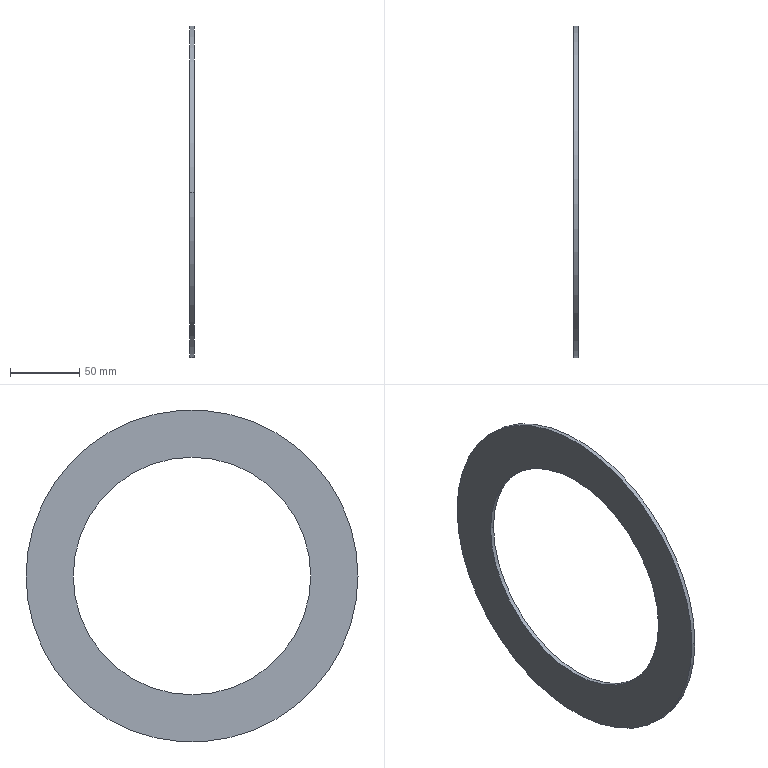Part | STEP file | 1 solid | 6 faces | box 3 x 239 x 239 mm | volume 65691 mm3 | cylinder 4 | plane 2 | commonest cylinder face diameters 171 x2 239 x2
STEP:
#1=CARTESIAN_POINT('',(0.,0.,0.));
#2=DIRECTION('',(0.,0.,1.));
#3=DIRECTION('',(1.,0.,0.));
#4=AXIS2_PLACEMENT_3D('',#1,#2,#3);
#5=CARTESIAN_POINT('',(3.,-85.5,0.));
#6=VERTEX_POINT('',#5);
#7=CARTESIAN_POINT('',(0.,-85.5,0.));
#8=VERTEX_POINT('',#7);
#9=CARTESIAN_POINT('',(0.,-85.5,0.));
#10=DIRECTION('',(-1.,0.,0.));
#11=VECTOR('',#10,1.);
#12=LINE('',#9,#11);
#13=CARTESIAN_POINT('',(0.,0.,0.));
#14=DIRECTION('',(-1.,0.,0.));
#15=DIRECTION('',(0.,-1.,0.));
#16=AXIS2_PLACEMENT_3D('',#13,#14,#15);
#17=CYLINDRICAL_SURFACE('',#16,85.5);
#18=CARTESIAN_POINT('',(6.283,0.));
#19=DIRECTION('',(0.,1.));
#20=VECTOR('',#19,1.);
#21=LINE('',#18,#20);
#22=(GEOMETRIC_REPRESENTATION_CONTEXT(2)PARAMETRIC_REPRESENTATION_CONTEXT()REPRESENTATION_CONTEXT('',''));
#23=DEFINITIONAL_REPRESENTATION('',(#21),#22);
#24=PCURVE('',#17,#23);
#25=CARTESIAN_POINT('',(0.,0.,0.));
#26=DIRECTION('',(-1.,0.,0.));
#27=DIRECTION('',(0.,-1.,0.));
#28=AXIS2_PLACEMENT_3D('',#25,#26,#27);
#29=CYLINDRICAL_SURFACE('',#28,85.5);
#30=CARTESIAN_POINT('',(0.,0.));
#31=DIRECTION('',(0.,1.));
#32=VECTOR('',#31,1.);
#33=LINE('',#30,#32);
#34=(GEOMETRIC_REPRESENTATION_CONTEXT(2)PARAMETRIC_REPRESENTATION_CONTEXT()REPRESENTATION_CONTEXT('',''));
#35=DEFINITIONAL_REPRESENTATION('',(#33),#34);
#36=PCURVE('',#29,#35);
#37=SURFACE_CURVE('',#12,(#24,#36),.PCURVE_S1.);
#38=EDGE_CURVE('',#6,#8,#37,.T.);
#39=ORIENTED_EDGE('',*,*,#38,.T.);
#40=CARTESIAN_POINT('',(0.,85.5,0.));
#41=VERTEX_POINT('',#40);
#42=CARTESIAN_POINT('',(0.,0.,0.));
#43=DIRECTION('',(-1.,0.,0.));
#44=DIRECTION('',(0.,-1.,0.));
#45=AXIS2_PLACEMENT_3D('',#42,#43,#44);
#46=CIRCLE('',#45,85.5);
#47=CARTESIAN_POINT('',(0.,0.));
#48=DIRECTION('',(1.,0.));
#49=VECTOR('',#48,1.);
#50=LINE('',#47,#49);
#51=(GEOMETRIC_REPRESENTATION_CONTEXT(2)PARAMETRIC_REPRESENTATION_CONTEXT()REPRESENTATION_CONTEXT('',''));
#52=DEFINITIONAL_REPRESENTATION('',(#50),#51);
#53=PCURVE('',#17,#52);
#54=CARTESIAN_POINT('',(0.,119.5,0.));
#55=DIRECTION('',(1.,0.,0.));
#56=DIRECTION('',(0.,1.,0.));
#57=AXIS2_PLACEMENT_3D('',#54,#55,#56);
#58=PLANE('',#57);
#59=CARTESIAN_POINT('',(-205.,0.));
#60=CARTESIAN_POINT('',(-205.,148.09));
#61=CARTESIAN_POINT('',(-76.75,74.045));
#62=CARTESIAN_POINT('',(51.5,0.));
#63=CARTESIAN_POINT('',(-76.75,-74.045));
#64=CARTESIAN_POINT('',(-205.,-148.09));
#65=CARTESIAN_POINT('',(-205.,0.));
#66=(BOUNDED_CURVE()B_SPLINE_CURVE(2,(#59,#60,#61,#62,#63,#64,#65),.UNSPECIFIED.,.T.,.F.)B_SPLINE_CURVE_WITH_KNOTS((1,2,2,2,2,1),(-2.094,0.,2.094,4.189,6.283,8.378),.UNSPECIFIED.)CURVE()GEOMETRIC_REPRESENTATION_ITEM()RATIONAL_B_SPLINE_CURVE((1.,0.5,1.,0.5,1.,0.5,1.))REPRESENTATION_ITEM(''));
#67=(GEOMETRIC_REPRESENTATION_CONTEXT(2)PARAMETRIC_REPRESENTATION_CONTEXT()REPRESENTATION_CONTEXT('',''));
#68=DEFINITIONAL_REPRESENTATION('',(#66),#67);
#69=PCURVE('',#58,#68);
#70=SURFACE_CURVE('',#46,(#53,#69),.PCURVE_S1.);
#71=EDGE_CURVE('',#41,#8,#70,.T.);
#72=ORIENTED_EDGE('',*,*,#71,.F.);
#73=CARTESIAN_POINT('',(3.,85.5,0.));
#74=VERTEX_POINT('',#73);
#75=CARTESIAN_POINT('',(0.,85.5,0.));
#76=DIRECTION('',(-1.,0.,0.));
#77=VECTOR('',#76,1.);
#78=LINE('',#75,#77);
#79=CARTESIAN_POINT('',(3.142,0.));
#80=DIRECTION('',(0.,1.));
#81=VECTOR('',#80,1.);
#82=LINE('',#79,#81);
#83=(GEOMETRIC_REPRESENTATION_CONTEXT(2)PARAMETRIC_REPRESENTATION_CONTEXT()REPRESENTATION_CONTEXT('',''));
#84=DEFINITIONAL_REPRESENTATION('',(#82),#83);
#85=PCURVE('',#17,#84);
#86=CARTESIAN_POINT('',(3.142,0.));
#87=DIRECTION('',(0.,1.));
#88=VECTOR('',#87,1.);
#89=LINE('',#86,#88);
#90=(GEOMETRIC_REPRESENTATION_CONTEXT(2)PARAMETRIC_REPRESENTATION_CONTEXT()REPRESENTATION_CONTEXT('',''));
#91=DEFINITIONAL_REPRESENTATION('',(#89),#90);
#92=PCURVE('',#29,#91);
#93=SURFACE_CURVE('',#78,(#85,#92),.PCURVE_S1.);
#94=EDGE_CURVE('',#74,#41,#93,.T.);
#95=ORIENTED_EDGE('',*,*,#94,.F.);
#96=CARTESIAN_POINT('',(3.,0.,0.));
#97=DIRECTION('',(-1.,0.,0.));
#98=DIRECTION('',(0.,-1.,0.));
#99=AXIS2_PLACEMENT_3D('',#96,#97,#98);
#100=CIRCLE('',#99,85.5);
#101=CARTESIAN_POINT('',(0.,-3.));
#102=DIRECTION('',(1.,0.));
#103=VECTOR('',#102,1.);
#104=LINE('',#101,#103);
#105=(GEOMETRIC_REPRESENTATION_CONTEXT(2)PARAMETRIC_REPRESENTATION_CONTEXT()REPRESENTATION_CONTEXT('',''));
#106=DEFINITIONAL_REPRESENTATION('',(#104),#105);
#107=PCURVE('',#17,#106);
#108=CARTESIAN_POINT('',(3.,85.5,0.));
#109=DIRECTION('',(-1.,0.,0.));
#110=DIRECTION('',(0.,-1.,0.));
#111=AXIS2_PLACEMENT_3D('',#108,#109,#110);
#112=PLANE('',#111);
#113=CARTESIAN_POINT('',(85.5,0.));
#114=DIRECTION('',(1.,0.));
#115=AXIS2_PLACEMENT_2D('',#113,#114);
#116=CIRCLE('',#115,85.5);
#117=(GEOMETRIC_REPRESENTATION_CONTEXT(2)PARAMETRIC_REPRESENTATION_CONTEXT()REPRESENTATION_CONTEXT('',''));
#118=DEFINITIONAL_REPRESENTATION('',(#116),#117);
#119=PCURVE('',#112,#118);
#120=SURFACE_CURVE('',#100,(#107,#119),.PCURVE_S1.);
#121=EDGE_CURVE('',#74,#6,#120,.T.);
#122=ORIENTED_EDGE('',*,*,#121,.T.);
#123=EDGE_LOOP('',(#39,#72,#95,#122));
#124=FACE_BOUND('',#123,.F.);
#125=ADVANCED_FACE('',(#124),#17,.F.);
#126=CARTESIAN_POINT('',(3.,-119.5,0.));
#127=VERTEX_POINT('',#126);
#128=CARTESIAN_POINT('',(3.,119.5,0.));
#129=VERTEX_POINT('',#128);
#130=CARTESIAN_POINT('',(3.,0.,0.));
#131=DIRECTION('',(-1.,0.,0.));
#132=DIRECTION('',(0.,-1.,0.));
#133=AXIS2_PLACEMENT_3D('',#130,#131,#132);
#134=CIRCLE('',#133,119.5);
#135=CARTESIAN_POINT('',(0.,0.,0.));
#136=DIRECTION('',(-1.,0.,0.));
#137=DIRECTION('',(0.,-1.,0.));
#138=AXIS2_PLACEMENT_3D('',#135,#136,#137);
#139=CYLINDRICAL_SURFACE('',#138,119.5);
#140=CARTESIAN_POINT('',(0.,-3.));
#141=DIRECTION('',(1.,0.));
#142=VECTOR('',#141,1.);
#143=LINE('',#140,#142);
#144=(GEOMETRIC_REPRESENTATION_CONTEXT(2)PARAMETRIC_REPRESENTATION_CONTEXT()REPRESENTATION_CONTEXT('',''));
#145=DEFINITIONAL_REPRESENTATION('',(#143),#144);
#146=PCURVE('',#139,#145);
#147=CARTESIAN_POINT('',(85.5,0.));
#148=DIRECTION('',(1.,0.));
#149=AXIS2_PLACEMENT_2D('',#147,#148);
#150=CIRCLE('',#149,119.5);
#151=(GEOMETRIC_REPRESENTATION_CONTEXT(2)PARAMETRIC_REPRESENTATION_CONTEXT()REPRESENTATION_CONTEXT('',''));
#152=DEFINITIONAL_REPRESENTATION('',(#150),#151);
#153=PCURVE('',#112,#152);
#154=SURFACE_CURVE('',#134,(#146,#153),.PCURVE_S1.);
#155=EDGE_CURVE('',#127,#129,#154,.T.);
#156=ORIENTED_EDGE('',*,*,#155,.T.);
#157=CARTESIAN_POINT('',(0.,119.5,0.));
#158=VERTEX_POINT('',#157);
#159=CARTESIAN_POINT('',(0.,119.5,0.));
#160=DIRECTION('',(-1.,0.,0.));
#161=VECTOR('',#160,1.);
#162=LINE('',#159,#161);
#163=CARTESIAN_POINT('',(3.142,0.));
#164=DIRECTION('',(0.,1.));
#165=VECTOR('',#164,1.);
#166=LINE('',#163,#165);
#167=(GEOMETRIC_REPRESENTATION_CONTEXT(2)PARAMETRIC_REPRESENTATION_CONTEXT()REPRESENTATION_CONTEXT('',''));
#168=DEFINITIONAL_REPRESENTATION('',(#166),#167);
#169=PCURVE('',#139,#168);
#170=CARTESIAN_POINT('',(0.,0.,0.));
#171=DIRECTION('',(-1.,0.,0.));
#172=DIRECTION('',(0.,-1.,0.));
#173=AXIS2_PLACEMENT_3D('',#170,#171,#172);
#174=CYLINDRICAL_SURFACE('',#173,119.5);
#175=CARTESIAN_POINT('',(3.142,0.));
#176=DIRECTION('',(0.,1.));
#177=VECTOR('',#176,1.);
#178=LINE('',#175,#177);
#179=(GEOMETRIC_REPRESENTATION_CONTEXT(2)PARAMETRIC_REPRESENTATION_CONTEXT()REPRESENTATION_CONTEXT('',''));
#180=DEFINITIONAL_REPRESENTATION('',(#178),#179);
#181=PCURVE('',#174,#180);
#182=SURFACE_CURVE('',#162,(#169,#181),.PCURVE_S1.);
#183=EDGE_CURVE('',#129,#158,#182,.T.);
#184=ORIENTED_EDGE('',*,*,#183,.T.);
#185=CARTESIAN_POINT('',(0.,-119.5,0.));
#186=VERTEX_POINT('',#185);
#187=CARTESIAN_POINT('',(0.,0.,0.));
#188=DIRECTION('',(-1.,0.,0.));
#189=DIRECTION('',(0.,-1.,0.));
#190=AXIS2_PLACEMENT_3D('',#187,#188,#189);
#191=CIRCLE('',#190,119.5);
#192=CARTESIAN_POINT('',(0.,0.));
#193=DIRECTION('',(1.,0.));
#194=VECTOR('',#193,1.);
#195=LINE('',#192,#194);
#196=(GEOMETRIC_REPRESENTATION_CONTEXT(2)PARAMETRIC_REPRESENTATION_CONTEXT()REPRESENTATION_CONTEXT('',''));
#197=DEFINITIONAL_REPRESENTATION('',(#195),#196);
#198=PCURVE('',#139,#197);
#199=CARTESIAN_POINT('',(-239.,0.));
#200=CARTESIAN_POINT('',(-239.,206.98));
#201=CARTESIAN_POINT('',(-59.75,103.49));
#202=CARTESIAN_POINT('',(119.5,0.));
#203=CARTESIAN_POINT('',(-59.75,-103.49));
#204=CARTESIAN_POINT('',(-239.,-206.98));
#205=CARTESIAN_POINT('',(-239.,0.));
#206=(BOUNDED_CURVE()B_SPLINE_CURVE(2,(#199,#200,#201,#202,#203,#204,#205),.UNSPECIFIED.,.T.,.F.)B_SPLINE_CURVE_WITH_KNOTS((1,2,2,2,2,1),(-2.094,0.,2.094,4.189,6.283,8.378),.UNSPECIFIED.)CURVE()GEOMETRIC_REPRESENTATION_ITEM()RATIONAL_B_SPLINE_CURVE((1.,0.5,1.,0.5,1.,0.5,1.))REPRESENTATION_ITEM(''));
#207=(GEOMETRIC_REPRESENTATION_CONTEXT(2)PARAMETRIC_REPRESENTATION_CONTEXT()REPRESENTATION_CONTEXT('',''));
#208=DEFINITIONAL_REPRESENTATION('',(#206),#207);
#209=PCURVE('',#58,#208);
#210=SURFACE_CURVE('',#191,(#198,#209),.PCURVE_S1.);
#211=EDGE_CURVE('',#186,#158,#210,.T.);
#212=ORIENTED_EDGE('',*,*,#211,.F.);
#213=CARTESIAN_POINT('',(0.,-119.5,0.));
#214=DIRECTION('',(-1.,0.,0.));
#215=VECTOR('',#214,1.);
#216=LINE('',#213,#215);
#217=CARTESIAN_POINT('',(0.,0.));
#218=DIRECTION('',(0.,1.));
#219=VECTOR('',#218,1.);
#220=LINE('',#217,#219);
#221=(GEOMETRIC_REPRESENTATION_CONTEXT(2)PARAMETRIC_REPRESENTATION_CONTEXT()REPRESENTATION_CONTEXT('',''));
#222=DEFINITIONAL_REPRESENTATION('',(#220),#221);
#223=PCURVE('',#139,#222);
#224=CARTESIAN_POINT('',(6.283,0.));
#225=DIRECTION('',(0.,1.));
#226=VECTOR('',#225,1.);
#227=LINE('',#224,#226);
#228=(GEOMETRIC_REPRESENTATION_CONTEXT(2)PARAMETRIC_REPRESENTATION_CONTEXT()REPRESENTATION_CONTEXT('',''));
#229=DEFINITIONAL_REPRESENTATION('',(#227),#228);
#230=PCURVE('',#174,#229);
#231=SURFACE_CURVE('',#216,(#223,#230),.PCURVE_S1.);
#232=EDGE_CURVE('',#127,#186,#231,.T.);
#233=ORIENTED_EDGE('',*,*,#232,.F.);
#234=EDGE_LOOP('',(#156,#184,#212,#233));
#235=FACE_BOUND('',#234,.T.);
#236=ADVANCED_FACE('',(#235),#139,.T.);
#237=ORIENTED_EDGE('',*,*,#183,.F.);
#238=CARTESIAN_POINT('',(3.,0.,0.));
#239=DIRECTION('',(-1.,0.,0.));
#240=DIRECTION('',(0.,-1.,0.));
#241=AXIS2_PLACEMENT_3D('',#238,#239,#240);
#242=CIRCLE('',#241,119.5);
#243=CARTESIAN_POINT('',(0.,-3.));
#244=DIRECTION('',(1.,0.));
#245=VECTOR('',#244,1.);
#246=LINE('',#243,#245);
#247=(GEOMETRIC_REPRESENTATION_CONTEXT(2)PARAMETRIC_REPRESENTATION_CONTEXT()REPRESENTATION_CONTEXT('',''));
#248=DEFINITIONAL_REPRESENTATION('',(#246),#247);
#249=PCURVE('',#174,#248);
#250=CARTESIAN_POINT('',(85.5,0.));
#251=DIRECTION('',(1.,0.));
#252=AXIS2_PLACEMENT_2D('',#250,#251);
#253=CIRCLE('',#252,119.5);
#254=(GEOMETRIC_REPRESENTATION_CONTEXT(2)PARAMETRIC_REPRESENTATION_CONTEXT()REPRESENTATION_CONTEXT('',''));
#255=DEFINITIONAL_REPRESENTATION('',(#253),#254);
#256=PCURVE('',#112,#255);
#257=SURFACE_CURVE('',#242,(#249,#256),.PCURVE_S1.);
#258=EDGE_CURVE('',#129,#127,#257,.T.);
#259=ORIENTED_EDGE('',*,*,#258,.T.);
#260=ORIENTED_EDGE('',*,*,#232,.T.);
#261=CARTESIAN_POINT('',(0.,0.,0.));
#262=DIRECTION('',(-1.,0.,0.));
#263=DIRECTION('',(0.,-1.,0.));
#264=AXIS2_PLACEMENT_3D('',#261,#262,#263);
#265=CIRCLE('',#264,119.5);
#266=CARTESIAN_POINT('',(0.,0.));
#267=DIRECTION('',(1.,0.));
#268=VECTOR('',#267,1.);
#269=LINE('',#266,#268);
#270=(GEOMETRIC_REPRESENTATION_CONTEXT(2)PARAMETRIC_REPRESENTATION_CONTEXT()REPRESENTATION_CONTEXT('',''));
#271=DEFINITIONAL_REPRESENTATION('',(#269),#270);
#272=PCURVE('',#174,#271);
#273=CARTESIAN_POINT('',(-239.,0.));
#274=CARTESIAN_POINT('',(-239.,206.98));
#275=CARTESIAN_POINT('',(-59.75,103.49));
#276=CARTESIAN_POINT('',(119.5,0.));
#277=CARTESIAN_POINT('',(-59.75,-103.49));
#278=CARTESIAN_POINT('',(-239.,-206.98));
#279=CARTESIAN_POINT('',(-239.,0.));
#280=(BOUNDED_CURVE()B_SPLINE_CURVE(2,(#273,#274,#275,#276,#277,#278,#279),.UNSPECIFIED.,.T.,.F.)B_SPLINE_CURVE_WITH_KNOTS((1,2,2,2,2,1),(-2.094,0.,2.094,4.189,6.283,8.378),.UNSPECIFIED.)CURVE()GEOMETRIC_REPRESENTATION_ITEM()RATIONAL_B_SPLINE_CURVE((1.,0.5,1.,0.5,1.,0.5,1.))REPRESENTATION_ITEM(''));
#281=(GEOMETRIC_REPRESENTATION_CONTEXT(2)PARAMETRIC_REPRESENTATION_CONTEXT()REPRESENTATION_CONTEXT('',''));
#282=DEFINITIONAL_REPRESENTATION('',(#280),#281);
#283=PCURVE('',#58,#282);
#284=SURFACE_CURVE('',#265,(#272,#283),.PCURVE_S1.);
#285=EDGE_CURVE('',#158,#186,#284,.T.);
#286=ORIENTED_EDGE('',*,*,#285,.F.);
#287=EDGE_LOOP('',(#237,#259,#260,#286));
#288=FACE_BOUND('',#287,.T.);
#289=ADVANCED_FACE('',(#288),#174,.T.);
#290=CARTESIAN_POINT('',(0.,0.,0.));
#291=DIRECTION('',(-1.,0.,0.));
#292=DIRECTION('',(0.,-1.,0.));
#293=AXIS2_PLACEMENT_3D('',#290,#291,#292);
#294=CIRCLE('',#293,85.5);
#295=CARTESIAN_POINT('',(-205.,0.));
#296=CARTESIAN_POINT('',(-205.,148.09));
#297=CARTESIAN_POINT('',(-76.75,74.045));
#298=CARTESIAN_POINT('',(51.5,0.));
#299=CARTESIAN_POINT('',(-76.75,-74.045));
#300=CARTESIAN_POINT('',(-205.,-148.09));
#301=CARTESIAN_POINT('',(-205.,0.));
#302=(BOUNDED_CURVE()B_SPLINE_CURVE(2,(#295,#296,#297,#298,#299,#300,#301),.UNSPECIFIED.,.T.,.F.)B_SPLINE_CURVE_WITH_KNOTS((1,2,2,2,2,1),(-2.094,0.,2.094,4.189,6.283,8.378),.UNSPECIFIED.)CURVE()GEOMETRIC_REPRESENTATION_ITEM()RATIONAL_B_SPLINE_CURVE((1.,0.5,1.,0.5,1.,0.5,1.))REPRESENTATION_ITEM(''));
#303=(GEOMETRIC_REPRESENTATION_CONTEXT(2)PARAMETRIC_REPRESENTATION_CONTEXT()REPRESENTATION_CONTEXT('',''));
#304=DEFINITIONAL_REPRESENTATION('',(#302),#303);
#305=PCURVE('',#58,#304);
#306=CARTESIAN_POINT('',(0.,0.));
#307=DIRECTION('',(1.,0.));
#308=VECTOR('',#307,1.);
#309=LINE('',#306,#308);
#310=(GEOMETRIC_REPRESENTATION_CONTEXT(2)PARAMETRIC_REPRESENTATION_CONTEXT()REPRESENTATION_CONTEXT('',''));
#311=DEFINITIONAL_REPRESENTATION('',(#309),#310);
#312=PCURVE('',#29,#311);
#313=SURFACE_CURVE('',#294,(#305,#312),.PCURVE_S1.);
#314=EDGE_CURVE('',#8,#41,#313,.T.);
#315=ORIENTED_EDGE('',*,*,#314,.F.);
#316=ORIENTED_EDGE('',*,*,#71,.F.);
#317=EDGE_LOOP('',(#315,#316));
#318=FACE_BOUND('',#317,.T.);
#319=ORIENTED_EDGE('',*,*,#211,.T.);
#320=ORIENTED_EDGE('',*,*,#285,.T.);
#321=EDGE_LOOP('',(#319,#320));
#322=FACE_BOUND('',#321,.T.);
#323=ADVANCED_FACE('',(#318,#322),#58,.F.);
#324=ORIENTED_EDGE('',*,*,#314,.F.);
#325=ORIENTED_EDGE('',*,*,#38,.F.);
#326=CARTESIAN_POINT('',(3.,0.,0.));
#327=DIRECTION('',(-1.,0.,0.));
#328=DIRECTION('',(0.,-1.,0.));
#329=AXIS2_PLACEMENT_3D('',#326,#327,#328);
#330=CIRCLE('',#329,85.5);
#331=CARTESIAN_POINT('',(0.,-3.));
#332=DIRECTION('',(1.,0.));
#333=VECTOR('',#332,1.);
#334=LINE('',#331,#333);
#335=(GEOMETRIC_REPRESENTATION_CONTEXT(2)PARAMETRIC_REPRESENTATION_CONTEXT()REPRESENTATION_CONTEXT('',''));
#336=DEFINITIONAL_REPRESENTATION('',(#334),#335);
#337=PCURVE('',#29,#336);
#338=CARTESIAN_POINT('',(85.5,0.));
#339=DIRECTION('',(1.,0.));
#340=AXIS2_PLACEMENT_2D('',#338,#339);
#341=CIRCLE('',#340,85.5);
#342=(GEOMETRIC_REPRESENTATION_CONTEXT(2)PARAMETRIC_REPRESENTATION_CONTEXT()REPRESENTATION_CONTEXT('',''));
#343=DEFINITIONAL_REPRESENTATION('',(#341),#342);
#344=PCURVE('',#112,#343);
#345=SURFACE_CURVE('',#330,(#337,#344),.PCURVE_S1.);
#346=EDGE_CURVE('',#6,#74,#345,.T.);
#347=ORIENTED_EDGE('',*,*,#346,.T.);
#348=ORIENTED_EDGE('',*,*,#94,.T.);
#349=EDGE_LOOP('',(#324,#325,#347,#348));
#350=FACE_BOUND('',#349,.F.);
#351=ADVANCED_FACE('',(#350),#29,.F.);
#352=ORIENTED_EDGE('',*,*,#155,.F.);
#353=ORIENTED_EDGE('',*,*,#258,.F.);
#354=EDGE_LOOP('',(#352,#353));
#355=FACE_BOUND('',#354,.T.);
#356=ORIENTED_EDGE('',*,*,#346,.T.);
#357=ORIENTED_EDGE('',*,*,#121,.T.);
#358=EDGE_LOOP('',(#356,#357));
#359=FACE_BOUND('',#358,.T.);
#360=ADVANCED_FACE('',(#355,#359),#112,.F.);
#361=CLOSED_SHELL('',(#125,#236,#289,#323,#351,#360));
#362=MANIFOLD_SOLID_BREP('',#361);
#363=(LENGTH_UNIT()NAMED_UNIT(*)SI_UNIT(.MILLI.,.METRE.));
#364=UNCERTAINTY_MEASURE_WITH_UNIT(LENGTH_MEASURE(0.0000001),#363,'','');
#365=(NAMED_UNIT(*)PLANE_ANGLE_UNIT()SI_UNIT($,.RADIAN.));
#366=(NAMED_UNIT(*)SI_UNIT($,.STERADIAN.)SOLID_ANGLE_UNIT());
#367=(GEOMETRIC_REPRESENTATION_CONTEXT(3)GLOBAL_UNCERTAINTY_ASSIGNED_CONTEXT((#364))GLOBAL_UNIT_ASSIGNED_CONTEXT((#363,#365,#366))REPRESENTATION_CONTEXT('',''));
#368=ADVANCED_BREP_SHAPE_REPRESENTATION('',(#4,#362),#367);